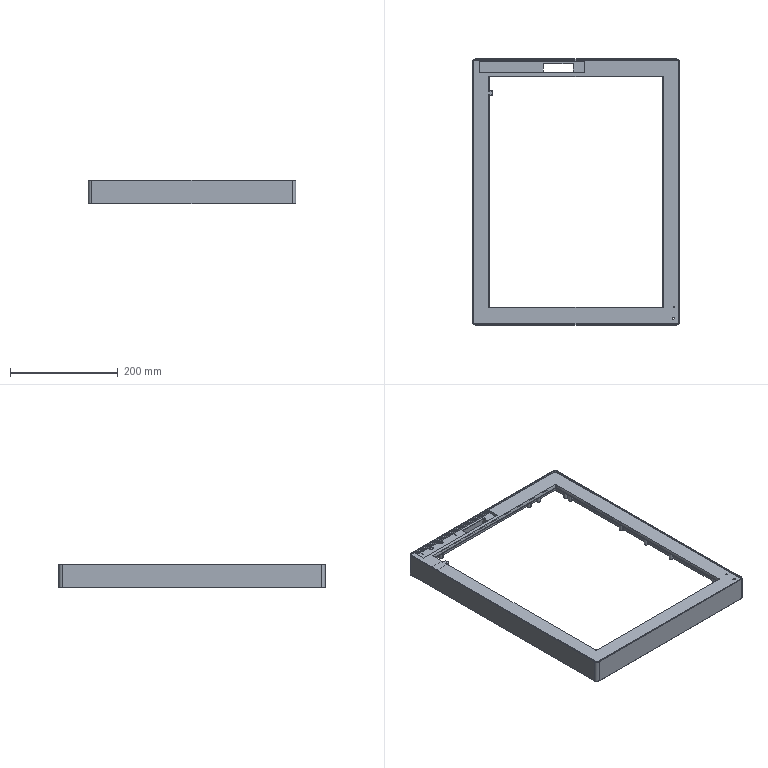Part | Creo | 1 solid | 1056 faces | box 384.532 x 492.964 x 44.276 mm | volume 412891 mm3 | plane 840 | cylinder 190 | torus 12 | cone 10 | spline 2 | sphere 2 | commonest cylinder face diameters 4.016 x46 8.032 x44 3.012 x33 10.04 x27 1 x8 34.412 x5